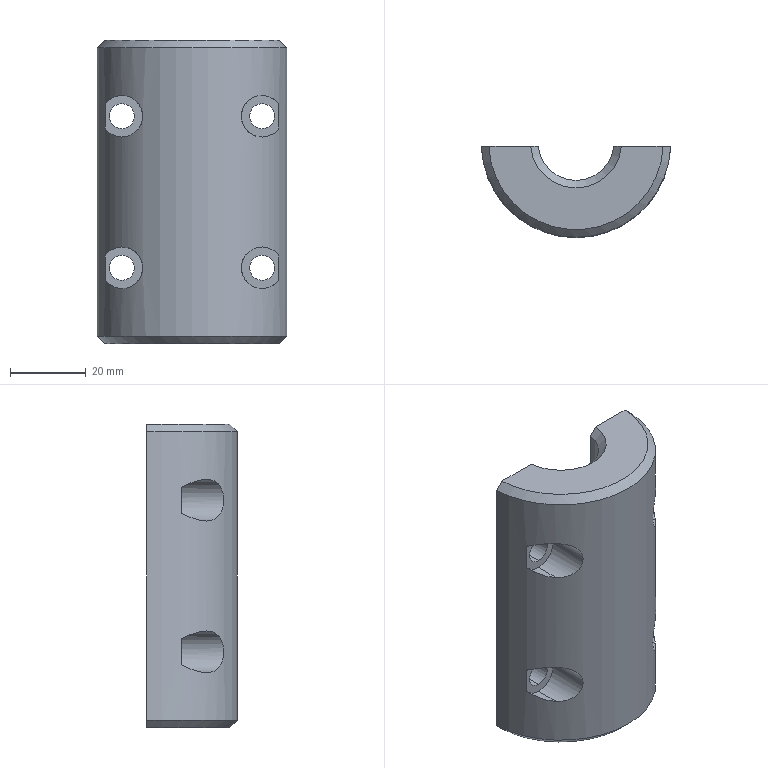Part | SolidWorks | features Chamfer 1, Extrusion 1, HoleWzd 1, ICE 1 | 1 solid | 34 faces | box 49.96 x 24 x 80 mm | volume 59562 mm3 | cylinder 22 | plane 8 | cone 4 | commonest cylinder face diameters 11 x12 6.6 x8 20 x1 50 x1
STEP:
#1=CARTESIAN_POINT('',(18.5,-1.,23.3));
#2=VERTEX_POINT('',#1);
#3=CARTESIAN_POINT('',(18.5,-1.,16.7));
#4=VERTEX_POINT('',#3);
#5=CARTESIAN_POINT('',(18.5,-1.,20.));
#6=DIRECTION('',(0.,-1.,0.));
#7=DIRECTION('',(0.,0.,-1.));
#8=AXIS2_PLACEMENT_3D('',#5,#6,#7);
#9=CIRCLE('',#8,3.3);
#10=EDGE_CURVE('',#2,#4,#9,.T.);
#11=ORIENTED_EDGE('',*,*,#10,.F.);
#12=CARTESIAN_POINT('',(18.5,-10.2,23.3));
#13=VERTEX_POINT('',#12);
#14=CARTESIAN_POINT('',(18.5,-17.,23.3));
#15=DIRECTION('',(0.,-1.,0.));
#16=VECTOR('',#15,1000.);
#17=LINE('',#14,#16);
#18=EDGE_CURVE('',#2,#13,#17,.T.);
#19=ORIENTED_EDGE('',*,*,#18,.T.);
#20=CARTESIAN_POINT('',(18.5,-10.2,16.7));
#21=VERTEX_POINT('',#20);
#22=CARTESIAN_POINT('',(18.5,-10.2,20.));
#23=DIRECTION('',(0.,-1.,0.));
#24=DIRECTION('',(0.,0.,-1.));
#25=AXIS2_PLACEMENT_3D('',#22,#23,#24);
#26=CIRCLE('',#25,3.3);
#27=EDGE_CURVE('',#13,#21,#26,.T.);
#28=ORIENTED_EDGE('',*,*,#27,.T.);
#29=CARTESIAN_POINT('',(18.5,-17.,16.7));
#30=DIRECTION('',(0.,-1.,0.));
#31=VECTOR('',#30,1000.);
#32=LINE('',#29,#31);
#33=EDGE_CURVE('',#4,#21,#32,.T.);
#34=ORIENTED_EDGE('',*,*,#33,.F.);
#35=EDGE_LOOP('',(#11,#19,#28,#34));
#36=FACE_OUTER_BOUND('',#35,.T.);
#37=CARTESIAN_POINT('',(18.5,-17.,20.));
#38=DIRECTION('',(0.,-1.,0.));
#39=DIRECTION('',(0.,0.,-1.));
#40=AXIS2_PLACEMENT_3D('',#37,#38,#39);
#41=CYLINDRICAL_SURFACE('',#40,3.3);
#42=ADVANCED_FACE('',(#36),#41,.F.);
#43=CARTESIAN_POINT('',(-18.5,-1.,23.3));
#44=VERTEX_POINT('',#43);
#45=CARTESIAN_POINT('',(-18.5,-1.,16.7));
#46=VERTEX_POINT('',#45);
#47=CARTESIAN_POINT('',(-18.5,-1.,20.));
#48=DIRECTION('',(0.,-1.,0.));
#49=DIRECTION('',(0.,0.,-1.));
#50=AXIS2_PLACEMENT_3D('',#47,#48,#49);
#51=CIRCLE('',#50,3.3);
#52=EDGE_CURVE('',#44,#46,#51,.T.);
#53=ORIENTED_EDGE('',*,*,#52,.F.);
#54=CARTESIAN_POINT('',(-18.5,-10.2,23.3));
#55=VERTEX_POINT('',#54);
#56=CARTESIAN_POINT('',(-18.5,-17.,23.3));
#57=DIRECTION('',(0.,-1.,0.));
#58=VECTOR('',#57,1000.);
#59=LINE('',#56,#58);
#60=EDGE_CURVE('',#44,#55,#59,.T.);
#61=ORIENTED_EDGE('',*,*,#60,.T.);
#62=CARTESIAN_POINT('',(-18.5,-10.2,16.7));
#63=VERTEX_POINT('',#62);
#64=CARTESIAN_POINT('',(-18.5,-10.2,20.));
#65=DIRECTION('',(0.,-1.,0.));
#66=DIRECTION('',(0.,0.,-1.));
#67=AXIS2_PLACEMENT_3D('',#64,#65,#66);
#68=CIRCLE('',#67,3.3);
#69=EDGE_CURVE('',#55,#63,#68,.T.);
#70=ORIENTED_EDGE('',*,*,#69,.T.);
#71=CARTESIAN_POINT('',(-18.5,-17.,16.7));
#72=DIRECTION('',(0.,-1.,0.));
#73=VECTOR('',#72,1000.);
#74=LINE('',#71,#73);
#75=EDGE_CURVE('',#46,#63,#74,.T.);
#76=ORIENTED_EDGE('',*,*,#75,.F.);
#77=EDGE_LOOP('',(#53,#61,#70,#76));
#78=FACE_OUTER_BOUND('',#77,.T.);
#79=CARTESIAN_POINT('',(-18.5,-17.,20.));
#80=DIRECTION('',(0.,-1.,0.));
#81=DIRECTION('',(0.,0.,-1.));
#82=AXIS2_PLACEMENT_3D('',#79,#80,#81);
#83=CYLINDRICAL_SURFACE('',#82,3.3);
#84=ADVANCED_FACE('',(#78),#83,.F.);
#85=CARTESIAN_POINT('',(-18.5,-1.,63.3));
#86=VERTEX_POINT('',#85);
#87=CARTESIAN_POINT('',(-18.5,-1.,56.7));
#88=VERTEX_POINT('',#87);
#89=CARTESIAN_POINT('',(-18.5,-1.,60.));
#90=DIRECTION('',(0.,-1.,0.));
#91=DIRECTION('',(0.,0.,-1.));
#92=AXIS2_PLACEMENT_3D('',#89,#90,#91);
#93=CIRCLE('',#92,3.3);
#94=EDGE_CURVE('',#86,#88,#93,.T.);
#95=ORIENTED_EDGE('',*,*,#94,.F.);
#96=CARTESIAN_POINT('',(-18.5,-10.2,63.3));
#97=VERTEX_POINT('',#96);
#98=CARTESIAN_POINT('',(-18.5,-17.,63.3));
#99=DIRECTION('',(0.,-1.,0.));
#100=VECTOR('',#99,1000.);
#101=LINE('',#98,#100);
#102=EDGE_CURVE('',#86,#97,#101,.T.);
#103=ORIENTED_EDGE('',*,*,#102,.T.);
#104=CARTESIAN_POINT('',(-18.5,-10.2,56.7));
#105=VERTEX_POINT('',#104);
#106=CARTESIAN_POINT('',(-18.5,-10.2,60.));
#107=DIRECTION('',(0.,-1.,0.));
#108=DIRECTION('',(0.,0.,-1.));
#109=AXIS2_PLACEMENT_3D('',#106,#107,#108);
#110=CIRCLE('',#109,3.3);
#111=EDGE_CURVE('',#97,#105,#110,.T.);
#112=ORIENTED_EDGE('',*,*,#111,.T.);
#113=CARTESIAN_POINT('',(-18.5,-17.,56.7));
#114=DIRECTION('',(0.,-1.,0.));
#115=VECTOR('',#114,1000.);
#116=LINE('',#113,#115);
#117=EDGE_CURVE('',#88,#105,#116,.T.);
#118=ORIENTED_EDGE('',*,*,#117,.F.);
#119=EDGE_LOOP('',(#95,#103,#112,#118));
#120=FACE_OUTER_BOUND('',#119,.T.);
#121=CARTESIAN_POINT('',(-18.5,-17.,60.));
#122=DIRECTION('',(0.,-1.,0.));
#123=DIRECTION('',(0.,0.,-1.));
#124=AXIS2_PLACEMENT_3D('',#121,#122,#123);
#125=CYLINDRICAL_SURFACE('',#124,3.3);
#126=ADVANCED_FACE('',(#120),#125,.F.);
#127=CARTESIAN_POINT('',(18.5,-1.,63.3));
#128=VERTEX_POINT('',#127);
#129=CARTESIAN_POINT('',(18.5,-1.,56.7));
#130=VERTEX_POINT('',#129);
#131=CARTESIAN_POINT('',(18.5,-1.,60.));
#132=DIRECTION('',(0.,-1.,0.));
#133=DIRECTION('',(0.,0.,-1.));
#134=AXIS2_PLACEMENT_3D('',#131,#132,#133);
#135=CIRCLE('',#134,3.3);
#136=EDGE_CURVE('',#128,#130,#135,.T.);
#137=ORIENTED_EDGE('',*,*,#136,.F.);
#138=CARTESIAN_POINT('',(18.5,-10.2,63.3));
#139=VERTEX_POINT('',#138);
#140=CARTESIAN_POINT('',(18.5,-17.,63.3));
#141=DIRECTION('',(0.,-1.,0.));
#142=VECTOR('',#141,1000.);
#143=LINE('',#140,#142);
#144=EDGE_CURVE('',#128,#139,#143,.T.);
#145=ORIENTED_EDGE('',*,*,#144,.T.);
#146=CARTESIAN_POINT('',(18.5,-10.2,56.7));
#147=VERTEX_POINT('',#146);
#148=CARTESIAN_POINT('',(18.5,-10.2,60.));
#149=DIRECTION('',(0.,-1.,0.));
#150=DIRECTION('',(0.,0.,-1.));
#151=AXIS2_PLACEMENT_3D('',#148,#149,#150);
#152=CIRCLE('',#151,3.3);
#153=EDGE_CURVE('',#139,#147,#152,.T.);
#154=ORIENTED_EDGE('',*,*,#153,.T.);
#155=CARTESIAN_POINT('',(18.5,-17.,56.7));
#156=DIRECTION('',(0.,-1.,0.));
#157=VECTOR('',#156,1000.);
#158=LINE('',#155,#157);
#159=EDGE_CURVE('',#130,#147,#158,.T.);
#160=ORIENTED_EDGE('',*,*,#159,.F.);
#161=EDGE_LOOP('',(#137,#145,#154,#160));
#162=FACE_OUTER_BOUND('',#161,.T.);
#163=CARTESIAN_POINT('',(18.5,-17.,60.));
#164=DIRECTION('',(0.,-1.,0.));
#165=DIRECTION('',(0.,0.,-1.));
#166=AXIS2_PLACEMENT_3D('',#163,#164,#165);
#167=CYLINDRICAL_SURFACE('',#166,3.3);
#168=ADVANCED_FACE('',(#162),#167,.F.);
#169=CARTESIAN_POINT('',(-18.5,-16.815,54.5));
#170=VERTEX_POINT('',#169);
#171=CARTESIAN_POINT('',(-22.825,-10.2,56.602));
#172=VERTEX_POINT('',#171);
#173=CARTESIAN_POINT('',(-18.5,-16.815,54.5));
#174=CARTESIAN_POINT('',(-18.967,-16.301,54.5));
#175=CARTESIAN_POINT('',(-19.407,-15.775,54.558));
#176=CARTESIAN_POINT('',(-20.028,-14.966,54.712));
#177=CARTESIAN_POINT('',(-20.229,-14.694,54.775));
#178=CARTESIAN_POINT('',(-20.618,-14.142,54.92));
#179=CARTESIAN_POINT('',(-20.808,-13.862,55.003));
#180=CARTESIAN_POINT('',(-21.352,-13.02,55.28));
#181=CARTESIAN_POINT('',(-21.685,-12.457,55.499));
#182=CARTESIAN_POINT('',(-22.295,-11.329,56.));
#183=CARTESIAN_POINT('',(-22.573,-10.763,56.281));
#184=CARTESIAN_POINT('',(-22.825,-10.2,56.602));
#185=B_SPLINE_CURVE_WITH_KNOTS('',3,(#173,#174,#175,#176,#177,#178,#179,#180,#181,#182,#183,#184),.UNSPECIFIED.,.F.,.F.,(4,2,2,2,2,4),(0.01974,0.02181,0.02284,0.02388,0.02594,0.02801),.UNSPECIFIED.);
#186=EDGE_CURVE('',#170,#172,#185,.T.);
#187=ORIENTED_EDGE('',*,*,#186,.F.);
#188=CARTESIAN_POINT('',(-18.5,-10.2,54.5));
#189=VERTEX_POINT('',#188);
#190=CARTESIAN_POINT('',(-18.5,-117.,54.5));
#191=DIRECTION('',(0.,1.,0.));
#192=VECTOR('',#191,1000.);
#193=LINE('',#190,#192);
#194=EDGE_CURVE('',#170,#189,#193,.T.);
#195=ORIENTED_EDGE('',*,*,#194,.T.);
#196=CARTESIAN_POINT('',(-18.5,-10.2,60.));
#197=DIRECTION('',(0.,-1.,0.));
#198=DIRECTION('',(0.,0.,-1.));
#199=AXIS2_PLACEMENT_3D('',#196,#197,#198);
#200=CIRCLE('',#199,5.5);
#201=EDGE_CURVE('',#172,#189,#200,.T.);
#202=ORIENTED_EDGE('',*,*,#201,.F.);
#203=EDGE_LOOP('',(#187,#195,#202));
#204=FACE_OUTER_BOUND('',#203,.T.);
#205=CARTESIAN_POINT('',(-18.5,-117.,60.));
#206=DIRECTION('',(0.,1.,0.));
#207=DIRECTION('',(0.,0.,1.));
#208=AXIS2_PLACEMENT_3D('',#205,#206,#207);
#209=CYLINDRICAL_SURFACE('',#208,5.5);
#210=ADVANCED_FACE('',(#204),#209,.F.);
#211=ORIENTED_EDGE('',*,*,#194,.F.);
#212=CARTESIAN_POINT('',(-18.5,-16.815,65.5));
#213=VERTEX_POINT('',#212);
#214=CARTESIAN_POINT('',(-18.5,-16.815,65.5));
#215=CARTESIAN_POINT('',(-18.218,-17.126,65.5));
#216=CARTESIAN_POINT('',(-17.927,-17.43,65.478));
#217=CARTESIAN_POINT('',(-17.34,-18.014,65.384));
#218=CARTESIAN_POINT('',(-17.042,-18.296,65.313));
#219=CARTESIAN_POINT('',(-16.439,-18.84,65.109));
#220=CARTESIAN_POINT('',(-16.133,-19.102,64.976));
#221=CARTESIAN_POINT('',(-15.538,-19.588,64.647));
#222=CARTESIAN_POINT('',(-15.248,-19.815,64.451));
#223=CARTESIAN_POINT('',(-14.828,-20.128,64.099));
#224=CARTESIAN_POINT('',(-14.691,-20.229,63.972));
#225=CARTESIAN_POINT('',(-14.429,-20.416,63.703));
#226=CARTESIAN_POINT('',(-14.304,-20.504,63.561));
#227=CARTESIAN_POINT('',(-14.066,-20.668,63.26));
#228=CARTESIAN_POINT('',(-13.953,-20.744,63.101));
#229=CARTESIAN_POINT('',(-13.741,-20.885,62.765));
#230=CARTESIAN_POINT('',(-13.643,-20.949,62.589));
#231=CARTESIAN_POINT('',(-13.379,-21.12,62.046));
#232=CARTESIAN_POINT('',(-13.241,-21.206,61.663));
#233=CARTESIAN_POINT('',(-13.098,-21.294,61.053));
#234=CARTESIAN_POINT('',(-13.061,-21.317,60.845));
#235=CARTESIAN_POINT('',(-13.013,-21.346,60.43));
#236=CARTESIAN_POINT('',(-13.001,-21.354,60.222));
#237=CARTESIAN_POINT('',(-12.999,-21.355,59.595));
#238=CARTESIAN_POINT('',(-13.047,-21.326,59.17));
#239=CARTESIAN_POINT('',(-13.187,-21.239,58.564));
#240=CARTESIAN_POINT('',(-13.244,-21.204,58.366));
#241=CARTESIAN_POINT('',(-13.381,-21.118,57.978));
#242=CARTESIAN_POINT('',(-13.461,-21.067,57.787));
#243=CARTESIAN_POINT('',(-13.725,-20.897,57.241));
#244=CARTESIAN_POINT('',(-13.936,-20.758,56.906));
#245=CARTESIAN_POINT('',(-14.417,-20.426,56.294));
#246=CARTESIAN_POINT('',(-14.68,-20.239,56.026));
#247=CARTESIAN_POINT('',(-15.098,-19.927,55.674));
#248=CARTESIAN_POINT('',(-15.242,-19.817,55.565));
#249=CARTESIAN_POINT('',(-15.534,-19.589,55.365));
#250=CARTESIAN_POINT('',(-15.682,-19.471,55.274));
#251=CARTESIAN_POINT('',(-16.127,-19.107,55.027));
#252=CARTESIAN_POINT('',(-16.427,-18.85,54.895));
#253=CARTESIAN_POINT('',(-17.032,-18.305,54.69));
#254=CARTESIAN_POINT('',(-17.335,-18.019,54.617));
#255=CARTESIAN_POINT('',(-17.926,-17.431,54.522));
#256=CARTESIAN_POINT('',(-18.217,-17.126,54.5));
#257=CARTESIAN_POINT('',(-18.5,-16.815,54.5));
#258=B_SPLINE_CURVE_WITH_KNOTS('',3,(#214,#215,#216,#217,#218,#219,#220,#221,#222,#223,#224,#225,#226,#227,#228,#229,#230,#231,#232,#233,#234,#235,#236,#237,#238,#239,#240,#241,#242,#243,#244,#245,#246,#247,#248,#249,#250,#251,#252,#253,#254,#255,#256,#257),.UNSPECIFIED.,.F.,.F.,(4,2,2,2,2,2,2,2,2,2,2,2,2,2,2,2,2,2,2,2,2,4),(-0.0002486,0.001001,0.00225,0.0035,0.004749,0.005374,0.005999,0.006623,0.007248,0.008497,0.009122,0.009747,0.011,0.01162,0.01225,0.0135,0.01474,0.01537,0.01599,0.01724,0.01849,0.01974),.UNSPECIFIED.);
#259=EDGE_CURVE('',#213,#170,#258,.T.);
#260=ORIENTED_EDGE('',*,*,#259,.F.);
#261=CARTESIAN_POINT('',(-18.5,-10.2,65.5));
#262=VERTEX_POINT('',#261);
#263=CARTESIAN_POINT('',(-18.5,-117.,65.5));
#264=DIRECTION('',(0.,1.,0.));
#265=VECTOR('',#264,1000.);
#266=LINE('',#263,#265);
#267=EDGE_CURVE('',#213,#262,#266,.T.);
#268=ORIENTED_EDGE('',*,*,#267,.T.);
#269=CARTESIAN_POINT('',(-18.5,-10.2,60.));
#270=DIRECTION('',(0.,-1.,0.));
#271=DIRECTION('',(0.,0.,-1.));
#272=AXIS2_PLACEMENT_3D('',#269,#270,#271);
#273=CIRCLE('',#272,5.5);
#274=EDGE_CURVE('',#189,#262,#273,.T.);
#275=ORIENTED_EDGE('',*,*,#274,.F.);
#276=EDGE_LOOP('',(#211,#260,#268,#275));
#277=FACE_OUTER_BOUND('',#276,.T.);
#278=CARTESIAN_POINT('',(-18.5,-117.,60.));
#279=DIRECTION('',(0.,1.,0.));
#280=DIRECTION('',(0.,0.,1.));
#281=AXIS2_PLACEMENT_3D('',#278,#279,#280);
#282=CYLINDRICAL_SURFACE('',#281,5.5);
#283=ADVANCED_FACE('',(#277),#282,.F.);
#284=CARTESIAN_POINT('',(18.5,-16.815,54.5));
#285=VERTEX_POINT('',#284);
#286=CARTESIAN_POINT('',(18.5,-16.815,65.5));
#287=VERTEX_POINT('',#286);
#288=CARTESIAN_POINT('',(18.5,-16.815,54.5));
#289=CARTESIAN_POINT('',(18.218,-17.126,54.5));
#290=CARTESIAN_POINT('',(17.927,-17.43,54.522));
#291=CARTESIAN_POINT('',(17.34,-18.014,54.616));
#292=CARTESIAN_POINT('',(17.042,-18.296,54.687));
#293=CARTESIAN_POINT('',(16.439,-18.84,54.891));
#294=CARTESIAN_POINT('',(16.133,-19.102,55.024));
#295=CARTESIAN_POINT('',(15.538,-19.588,55.353));
#296=CARTESIAN_POINT('',(15.248,-19.815,55.549));
#297=CARTESIAN_POINT('',(14.828,-20.128,55.901));
#298=CARTESIAN_POINT('',(14.691,-20.229,56.028));
#299=CARTESIAN_POINT('',(14.429,-20.416,56.297));
#300=CARTESIAN_POINT('',(14.304,-20.504,56.439));
#301=CARTESIAN_POINT('',(14.066,-20.668,56.74));
#302=CARTESIAN_POINT('',(13.953,-20.744,56.899));
#303=CARTESIAN_POINT('',(13.741,-20.885,57.235));
#304=CARTESIAN_POINT('',(13.643,-20.949,57.411));
#305=CARTESIAN_POINT('',(13.379,-21.12,57.954));
#306=CARTESIAN_POINT('',(13.241,-21.206,58.337));
#307=CARTESIAN_POINT('',(13.098,-21.294,58.947));
#308=CARTESIAN_POINT('',(13.061,-21.317,59.155));
#309=CARTESIAN_POINT('',(13.013,-21.346,59.57));
#310=CARTESIAN_POINT('',(13.001,-21.354,59.778));
#311=CARTESIAN_POINT('',(12.999,-21.355,60.405));
#312=CARTESIAN_POINT('',(13.047,-21.326,60.83));
#313=CARTESIAN_POINT('',(13.187,-21.239,61.436));
#314=CARTESIAN_POINT('',(13.244,-21.204,61.634));
#315=CARTESIAN_POINT('',(13.381,-21.118,62.022));
#316=CARTESIAN_POINT('',(13.461,-21.067,62.213));
#317=CARTESIAN_POINT('',(13.725,-20.897,62.759));
#318=CARTESIAN_POINT('',(13.936,-20.758,63.094));
#319=CARTESIAN_POINT('',(14.417,-20.426,63.706));
#320=CARTESIAN_POINT('',(14.68,-20.239,63.974));
#321=CARTESIAN_POINT('',(15.098,-19.927,64.326));
#322=CARTESIAN_POINT('',(15.242,-19.817,64.435));
#323=CARTESIAN_POINT('',(15.534,-19.589,64.635));
#324=CARTESIAN_POINT('',(15.682,-19.471,64.726));
#325=CARTESIAN_POINT('',(16.127,-19.107,64.973));
#326=CARTESIAN_POINT('',(16.427,-18.85,65.105));
#327=CARTESIAN_POINT('',(17.032,-18.305,65.31));
#328=CARTESIAN_POINT('',(17.335,-18.019,65.383));
#329=CARTESIAN_POINT('',(17.926,-17.431,65.478));
#330=CARTESIAN_POINT('',(18.217,-17.126,65.5));
#331=CARTESIAN_POINT('',(18.5,-16.815,65.5));
#332=B_SPLINE_CURVE_WITH_KNOTS('',3,(#288,#289,#290,#291,#292,#293,#294,#295,#296,#297,#298,#299,#300,#301,#302,#303,#304,#305,#306,#307,#308,#309,#310,#311,#312,#313,#314,#315,#316,#317,#318,#319,#320,#321,#322,#323,#324,#325,#326,#327,#328,#329,#330,#331),.UNSPECIFIED.,.F.,.F.,(4,2,2,2,2,2,2,2,2,2,2,2,2,2,2,2,2,2,2,2,2,4),(-0.0002486,0.001001,0.00225,0.0035,0.004749,0.005374,0.005999,0.006623,0.007248,0.008497,0.009122,0.009747,0.011,0.01162,0.01225,0.0135,0.01474,0.01537,0.01599,0.01724,0.01849,0.01974),.UNSPECIFIED.);
#333=EDGE_CURVE('',#285,#287,#332,.T.);
#334=ORIENTED_EDGE('',*,*,#333,.F.);
#335=CARTESIAN_POINT('',(18.5,-10.2,54.5));
#336=VERTEX_POINT('',#335);
#337=CARTESIAN_POINT('',(18.5,-117.,54.5));
#338=DIRECTION('',(0.,1.,0.));
#339=VECTOR('',#338,1000.);
#340=LINE('',#337,#339);
#341=EDGE_CURVE('',#285,#336,#340,.T.);
#342=ORIENTED_EDGE('',*,*,#341,.T.);
#343=CARTESIAN_POINT('',(18.5,-10.2,65.5));
#344=VERTEX_POINT('',#343);
#345=CARTESIAN_POINT('',(18.5,-10.2,60.));
#346=DIRECTION('',(0.,-1.,0.));
#347=DIRECTION('',(0.,0.,-1.));
#348=AXIS2_PLACEMENT_3D('',#345,#346,#347);
#349=CIRCLE('',#348,5.5);
#350=EDGE_CURVE('',#344,#336,#349,.T.);
#351=ORIENTED_EDGE('',*,*,#350,.F.);
#352=CARTESIAN_POINT('',(18.5,-117.,65.5));
#353=DIRECTION('',(0.,1.,0.));
#354=VECTOR('',#353,1000.);
#355=LINE('',#352,#354);
#356=EDGE_CURVE('',#287,#344,#355,.T.);
#357=ORIENTED_EDGE('',*,*,#356,.F.);
#358=EDGE_LOOP('',(#334,#342,#351,#357));
#359=FACE_OUTER_BOUND('',#358,.T.);
#360=CARTESIAN_POINT('',(18.5,-117.,60.));
#361=DIRECTION('',(0.,1.,0.));
#362=DIRECTION('',(0.,0.,1.));
#363=AXIS2_PLACEMENT_3D('',#360,#361,#362);
#364=CYLINDRICAL_SURFACE('',#363,5.5);
#365=ADVANCED_FACE('',(#359),#364,.F.);
#366=CARTESIAN_POINT('',(22.825,-10.2,63.398));
#367=VERTEX_POINT('',#366);
#368=CARTESIAN_POINT('',(18.5,-16.815,65.5));
#369=CARTESIAN_POINT('',(18.967,-16.301,65.5));
#370=CARTESIAN_POINT('',(19.407,-15.775,65.442));
#371=CARTESIAN_POINT('',(20.028,-14.966,65.288));
#372=CARTESIAN_POINT('',(20.229,-14.694,65.225));
#373=CARTESIAN_POINT('',(20.618,-14.142,65.08));
#374=CARTESIAN_POINT('',(20.808,-13.862,64.997));
#375=CARTESIAN_POINT('',(21.352,-13.02,64.72));
#376=CARTESIAN_POINT('',(21.685,-12.457,64.501));
#377=CARTESIAN_POINT('',(22.295,-11.329,64.));
#378=CARTESIAN_POINT('',(22.573,-10.763,63.719));
#379=CARTESIAN_POINT('',(22.825,-10.2,63.398));
#380=B_SPLINE_CURVE_WITH_KNOTS('',3,(#368,#369,#370,#371,#372,#373,#374,#375,#376,#377,#378,#379),.UNSPECIFIED.,.F.,.F.,(4,2,2,2,2,4),(0.01974,0.02181,0.02284,0.02388,0.02594,0.02801),.UNSPECIFIED.);
#381=EDGE_CURVE('',#287,#367,#380,.T.);
#382=ORIENTED_EDGE('',*,*,#381,.F.);
#383=ORIENTED_EDGE('',*,*,#356,.T.);
#384=CARTESIAN_POINT('',(18.5,-10.2,60.));
#385=DIRECTION('',(0.,-1.,0.));
#386=DIRECTION('',(0.,0.,-1.));
#387=AXIS2_PLACEMENT_3D('',#384,#385,#386);
#388=CIRCLE('',#387,5.5);
#389=EDGE_CURVE('',#367,#344,#388,.T.);
#390=ORIENTED_EDGE('',*,*,#389,.F.);
#391=EDGE_LOOP('',(#382,#383,#390));
#392=FACE_OUTER_BOUND('',#391,.T.);
#393=CARTESIAN_POINT('',(18.5,-117.,60.));
#394=DIRECTION('',(0.,1.,0.));
#395=DIRECTION('',(0.,0.,1.));
#396=AXIS2_PLACEMENT_3D('',#393,#394,#395);
#397=CYLINDRICAL_SURFACE('',#396,5.5);
#398=ADVANCED_FACE('',(#392),#397,.F.);
#399=CARTESIAN_POINT('',(18.5,-16.815,14.5));
#400=VERTEX_POINT('',#399);
#401=CARTESIAN_POINT('',(18.5,-16.815,25.5));
#402=VERTEX_POINT('',#401);
#403=CARTESIAN_POINT('',(18.5,-16.815,14.5));
#404=CARTESIAN_POINT('',(18.218,-17.126,14.5));
#405=CARTESIAN_POINT('',(17.927,-17.43,14.522));
#406=CARTESIAN_POINT('',(17.34,-18.014,14.616));
#407=CARTESIAN_POINT('',(17.042,-18.296,14.687));
#408=CARTESIAN_POINT('',(16.439,-18.84,14.891));
#409=CARTESIAN_POINT('',(16.133,-19.102,15.024));
#410=CARTESIAN_POINT('',(15.538,-19.588,15.353));
#411=CARTESIAN_POINT('',(15.248,-19.815,15.549));
#412=CARTESIAN_POINT('',(14.828,-20.128,15.901));
#413=CARTESIAN_POINT('',(14.691,-20.229,16.028));
#414=CARTESIAN_POINT('',(14.429,-20.416,16.297));
#415=CARTESIAN_POINT('',(14.304,-20.504,16.439));
#416=CARTESIAN_POINT('',(14.066,-20.668,16.74));
#417=CARTESIAN_POINT('',(13.953,-20.744,16.899));
#418=CARTESIAN_POINT('',(13.741,-20.885,17.235));
#419=CARTESIAN_POINT('',(13.643,-20.949,17.411));
#420=CARTESIAN_POINT('',(13.379,-21.12,17.954));
#421=CARTESIAN_POINT('',(13.241,-21.206,18.337));
#422=CARTESIAN_POINT('',(13.098,-21.294,18.947));
#423=CARTESIAN_POINT('',(13.061,-21.317,19.155));
#424=CARTESIAN_POINT('',(13.013,-21.346,19.57));
#425=CARTESIAN_POINT('',(13.001,-21.354,19.778));
#426=CARTESIAN_POINT('',(12.999,-21.355,20.405));
#427=CARTESIAN_POINT('',(13.047,-21.326,20.83));
#428=CARTESIAN_POINT('',(13.187,-21.239,21.436));
#429=CARTESIAN_POINT('',(13.244,-21.204,21.634));
#430=CARTESIAN_POINT('',(13.381,-21.118,22.022));
#431=CARTESIAN_POINT('',(13.461,-21.067,22.213));
#432=CARTESIAN_POINT('',(13.725,-20.897,22.759));
#433=CARTESIAN_POINT('',(13.936,-20.758,23.094));
#434=CARTESIAN_POINT('',(14.417,-20.426,23.706));
#435=CARTESIAN_POINT('',(14.68,-20.239,23.974));
#436=CARTESIAN_POINT('',(15.098,-19.927,24.326));
#437=CARTESIAN_POINT('',(15.242,-19.817,24.435));
#438=CARTESIAN_POINT('',(15.534,-19.589,24.635));
#439=CARTESIAN_POINT('',(15.682,-19.471,24.726));
#440=CARTESIAN_POINT('',(16.127,-19.107,24.973));
#441=CARTESIAN_POINT('',(16.427,-18.85,25.105));
#442=CARTESIAN_POINT('',(17.032,-18.305,25.31));
#443=CARTESIAN_POINT('',(17.335,-18.019,25.383));
#444=CARTESIAN_POINT('',(17.926,-17.431,25.478));
#445=CARTESIAN_POINT('',(18.217,-17.126,25.5));
#446=CARTESIAN_POINT('',(18.5,-16.815,25.5));
#447=B_SPLINE_CURVE_WITH_KNOTS('',3,(#403,#404,#405,#406,#407,#408,#409,#410,#411,#412,#413,#414,#415,#416,#417,#418,#419,#420,#421,#422,#423,#424,#425,#426,#427,#428,#429,#430,#431,#432,#433,#434,#435,#436,#437,#438,#439,#440,#441,#442,#443,#444,#445,#446),.UNSPECIFIED.,.F.,.F.,(4,2,2,2,2,2,2,2,2,2,2,2,2,2,2,2,2,2,2,2,2,4),(-0.0002486,0.001001,0.00225,0.0035,0.004749,0.005374,0.005999,0.006623,0.007248,0.008497,0.009122,0.009747,0.011,0.01162,0.01225,0.0135,0.01474,0.01537,0.01599,0.01724,0.01849,0.01974),.UNSPECIFIED.);
#448=EDGE_CURVE('',#400,#402,#447,.T.);
#449=ORIENTED_EDGE('',*,*,#448,.F.);
#450=CARTESIAN_POINT('',(18.5,-10.2,14.5));
#451=VERTEX_POINT('',#450);
#452=CARTESIAN_POINT('',(18.5,-117.,14.5));
#453=DIRECTION('',(0.,1.,0.));
#454=VECTOR('',#453,1000.);
#455=LINE('',#452,#454);
#456=EDGE_CURVE('',#400,#451,#455,.T.);
#457=ORIENTED_EDGE('',*,*,#456,.T.);
#458=CARTESIAN_POINT('',(18.5,-10.2,25.5));
#459=VERTEX_POINT('',#458);
#460=CARTESIAN_POINT('',(18.5,-10.2,20.));
#461=DIRECTION('',(0.,-1.,0.));
#462=DIRECTION('',(0.,0.,-1.));
#463=AXIS2_PLACEMENT_3D('',#460,#461,#462);
#464=CIRCLE('',#463,5.5);
#465=EDGE_CURVE('',#459,#451,#464,.T.);
#466=ORIENTED_EDGE('',*,*,#465,.F.);
#467=CARTESIAN_POINT('',(18.5,-117.,25.5));
#468=DIRECTION('',(0.,1.,0.));
#469=VECTOR('',#468,1000.);
#470=LINE('',#467,#469);
#471=EDGE_CURVE('',#402,#459,#470,.T.);
#472=ORIENTED_EDGE('',*,*,#471,.F.);
#473=EDGE_LOOP('',(#449,#457,#466,#472));
#474=FACE_OUTER_BOUND('',#473,.T.);
#475=CARTESIAN_POINT('',(18.5,-117.,20.));
#476=DIRECTION('',(0.,1.,0.));
#477=DIRECTION('',(0.,0.,1.));
#478=AXIS2_PLACEMENT_3D('',#475,#476,#477);
#479=CYLINDRICAL_SURFACE('',#478,5.5);
#480=ADVANCED_FACE('',(#474),#479,.F.);
#481=CARTESIAN_POINT('',(22.825,-10.2,23.398));
#482=VERTEX_POINT('',#481);
#483=CARTESIAN_POINT('',(18.5,-16.815,25.5));
#484=CARTESIAN_POINT('',(18.967,-16.301,25.5));
#485=CARTESIAN_POINT('',(19.407,-15.775,25.442));
#486=CARTESIAN_POINT('',(20.028,-14.966,25.288));
#487=CARTESIAN_POINT('',(20.229,-14.694,25.225));
#488=CARTESIAN_POINT('',(20.618,-14.142,25.08));
#489=CARTESIAN_POINT('',(20.808,-13.862,24.997));
#490=CARTESIAN_POINT('',(21.352,-13.02,24.72));
#491=CARTESIAN_POINT('',(21.685,-12.457,24.501));
#492=CARTESIAN_POINT('',(22.295,-11.329,24.));
#493=CARTESIAN_POINT('',(22.573,-10.763,23.719));
#494=CARTESIAN_POINT('',(22.825,-10.2,23.398));
#495=B_SPLINE_CURVE_WITH_KNOTS('',3,(#483,#484,#485,#486,#487,#488,#489,#490,#491,#492,#493,#494),.UNSPECIFIED.,.F.,.F.,(4,2,2,2,2,4),(0.01974,0.02181,0.02284,0.02388,0.02594,0.02801),.UNSPECIFIED.);
#496=EDGE_CURVE('',#402,#482,#495,.T.);
#497=ORIENTED_EDGE('',*,*,#496,.F.);
#498=ORIENTED_EDGE('',*,*,#471,.T.);
#499=CARTESIAN_POINT('',(18.5,-10.2,20.));
#500=DIRECTION('',(0.,-1.,0.));
#501=DIRECTION('',(0.,0.,-1.));
#502=AXIS2_PLACEMENT_3D('',#499,#500,#501);
#503=CIRCLE('',#502,5.5);
#504=EDGE_CURVE('',#482,#459,#503,.T.);
#505=ORIENTED_EDGE('',*,*,#504,.F.);
#506=EDGE_LOOP('',(#497,#498,#505));
#507=FACE_OUTER_BOUND('',#506,.T.);
#508=CARTESIAN_POINT('',(18.5,-117.,20.));
#509=DIRECTION('',(0.,1.,0.));
#510=DIRECTION('',(0.,0.,1.));
#511=AXIS2_PLACEMENT_3D('',#508,#509,#510);
#512=CYLINDRICAL_SURFACE('',#511,5.5);
#513=ADVANCED_FACE('',(#507),#512,.F.);
#514=CARTESIAN_POINT('',(-18.5,-16.815,14.5));
#515=VERTEX_POINT('',#514);
#516=CARTESIAN_POINT('',(-22.825,-10.2,16.602));
#517=VERTEX_POINT('',#516);
#518=CARTESIAN_POINT('',(-18.5,-16.815,14.5));
#519=CARTESIAN_POINT('',(-18.967,-16.301,14.5));
#520=CARTESIAN_POINT('',(-19.407,-15.775,14.558));
#521=CARTESIAN_POINT('',(-20.028,-14.966,14.712));
#522=CARTESIAN_POINT('',(-20.229,-14.694,14.775));
#523=CARTESIAN_POINT('',(-20.618,-14.142,14.92));
#524=CARTESIAN_POINT('',(-20.808,-13.862,15.003));
#525=CARTESIAN_POINT('',(-21.352,-13.02,15.28));
#526=CARTESIAN_POINT('',(-21.685,-12.457,15.499));
#527=CARTESIAN_POINT('',(-22.295,-11.329,16.));
#528=CARTESIAN_POINT('',(-22.573,-10.763,16.281));
#529=CARTESIAN_POINT('',(-22.825,-10.2,16.602));
#530=B_SPLINE_CURVE_WITH_KNOTS('',3,(#518,#519,#520,#521,#522,#523,#524,#525,#526,#527,#528,#529),.UNSPECIFIED.,.F.,.F.,(4,2,2,2,2,4),(0.01974,0.02181,0.02284,0.02388,0.02594,0.02801),.UNSPECIFIED.);
#531=EDGE_CURVE('',#515,#517,#530,.T.);
#532=ORIENTED_EDGE('',*,*,#531,.F.);
#533=CARTESIAN_POINT('',(-18.5,-10.2,14.5));
#534=VERTEX_POINT('',#533);
#535=CARTESIAN_POINT('',(-18.5,-117.,14.5));
#536=DIRECTION('',(0.,1.,0.));
#537=VECTOR('',#536,1000.);
#538=LINE('',#535,#537);
#539=EDGE_CURVE('',#515,#534,#538,.T.);
#540=ORIENTED_EDGE('',*,*,#539,.T.);
#541=CARTESIAN_POINT('',(-18.5,-10.2,20.));
#542=DIRECTION('',(0.,-1.,0.));
#543=DIRECTION('',(0.,0.,-1.));
#544=AXIS2_PLACEMENT_3D('',#541,#542,#543);
#545=CIRCLE('',#544,5.5);
#546=EDGE_CURVE('',#517,#534,#545,.T.);
#547=ORIENTED_EDGE('',*,*,#546,.F.);
#548=EDGE_LOOP('',(#532,#540,#547));
#549=FACE_OUTER_BOUND('',#548,.T.);
#550=CARTESIAN_POINT('',(-18.5,-117.,20.));
#551=DIRECTION('',(0.,1.,0.));
#552=DIRECTION('',(0.,0.,1.));
#553=AXIS2_PLACEMENT_3D('',#550,#551,#552);
#554=CYLINDRICAL_SURFACE('',#553,5.5);
#555=ADVANCED_FACE('',(#549),#554,.F.);
#556=ORIENTED_EDGE('',*,*,#539,.F.);
#557=CARTESIAN_POINT('',(-18.5,-16.815,25.5));
#558=VERTEX_POINT('',#557);
#559=CARTESIAN_POINT('',(-18.5,-16.815,25.5));
#560=CARTESIAN_POINT('',(-18.218,-17.126,25.5));
#561=CARTESIAN_POINT('',(-17.927,-17.43,25.478));
#562=CARTESIAN_POINT('',(-17.34,-18.014,25.384));
#563=CARTESIAN_POINT('',(-17.042,-18.296,25.313));
#564=CARTESIAN_POINT('',(-16.439,-18.84,25.109));
#565=CARTESIAN_POINT('',(-16.133,-19.102,24.976));
#566=CARTESIAN_POINT('',(-15.538,-19.588,24.647));
#567=CARTESIAN_POINT('',(-15.248,-19.815,24.451));
#568=CARTESIAN_POINT('',(-14.828,-20.128,24.099));
#569=CARTESIAN_POINT('',(-14.691,-20.229,23.972));
#570=CARTESIAN_POINT('',(-14.429,-20.416,23.703));
#571=CARTESIAN_POINT('',(-14.304,-20.504,23.561));
#572=CARTESIAN_POINT('',(-14.066,-20.668,23.26));
#573=CARTESIAN_POINT('',(-13.953,-20.744,23.101));
#574=CARTESIAN_POINT('',(-13.741,-20.885,22.765));
#575=CARTESIAN_POINT('',(-13.643,-20.949,22.589));
#576=CARTESIAN_POINT('',(-13.379,-21.12,22.046));
#577=CARTESIAN_POINT('',(-13.241,-21.206,21.663));
#578=CARTESIAN_POINT('',(-13.098,-21.294,21.053));
#579=CARTESIAN_POINT('',(-13.061,-21.317,20.845));
#580=CARTESIAN_POINT('',(-13.013,-21.346,20.43));
#581=CARTESIAN_POINT('',(-13.001,-21.354,20.222));
#582=CARTESIAN_POINT('',(-12.999,-21.355,19.595));
#583=CARTESIAN_POINT('',(-13.047,-21.326,19.17));
#584=CARTESIAN_POINT('',(-13.187,-21.239,18.564));
#585=CARTESIAN_POINT('',(-13.244,-21.204,18.366));
#586=CARTESIAN_POINT('',(-13.381,-21.118,17.978));
#587=CARTESIAN_POINT('',(-13.461,-21.067,17.787));
#588=CARTESIAN_POINT('',(-13.725,-20.897,17.241));
#589=CARTESIAN_POINT('',(-13.936,-20.758,16.906));
#590=CARTESIAN_POINT('',(-14.417,-20.426,16.294));
#591=CARTESIAN_POINT('',(-14.68,-20.239,16.026));
#592=CARTESIAN_POINT('',(-15.098,-19.927,15.674));
#593=CARTESIAN_POINT('',(-15.242,-19.817,15.565));
#594=CARTESIAN_POINT('',(-15.534,-19.589,15.365));
#595=CARTESIAN_POINT('',(-15.682,-19.471,15.274));
#596=CARTESIAN_POINT('',(-16.127,-19.107,15.027));
#597=CARTESIAN_POINT('',(-16.427,-18.85,14.895));
#598=CARTESIAN_POINT('',(-17.032,-18.305,14.69));
#599=CARTESIAN_POINT('',(-17.335,-18.019,14.617));
#600=CARTESIAN_POINT('',(-17.926,-17.431,14.522));
#601=CARTESIAN_POINT('',(-18.217,-17.126,14.5));
#602=CARTESIAN_POINT('',(-18.5,-16.815,14.5));
#603=B_SPLINE_CURVE_WITH_KNOTS('',3,(#559,#560,#561,#562,#563,#564,#565,#566,#567,#568,#569,#570,#571,#572,#573,#574,#575,#576,#577,#578,#579,#580,#581,#582,#583,#584,#585,#586,#587,#588,#589,#590,#591,#592,#593,#594,#595,#596,#597,#598,#599,#600,#601,#602),.UNSPECIFIED.,.F.,.F.,(4,2,2,2,2,2,2,2,2,2,2,2,2,2,2,2,2,2,2,2,2,4),(-0.0002486,0.001001,0.00225,0.0035,0.004749,0.005374,0.005999,0.006623,0.007248,0.008497,0.009122,0.009747,0.011,0.01162,0.01225,0.0135,0.01474,0.01537,0.01599,0.01724,0.01849,0.01974),.UNSPECIFIED.);
#604=EDGE_CURVE('',#558,#515,#603,.T.);
#605=ORIENTED_EDGE('',*,*,#604,.F.);
#606=CARTESIAN_POINT('',(-18.5,-10.2,25.5));
#607=VERTEX_POINT('',#606);
#608=CARTESIAN_POINT('',(-18.5,-117.,25.5));
#609=DIRECTION('',(0.,1.,0.));
#610=VECTOR('',#609,1000.);
#611=LINE('',#608,#610);
#612=EDGE_CURVE('',#558,#607,#611,.T.);
#613=ORIENTED_EDGE('',*,*,#612,.T.);
#614=CARTESIAN_POINT('',(-18.5,-10.2,20.));
#615=DIRECTION('',(0.,-1.,0.));
#616=DIRECTION('',(0.,0.,-1.));
#617=AXIS2_PLACEMENT_3D('',#614,#615,#616);
#618=CIRCLE('',#617,5.5);
#619=EDGE_CURVE('',#534,#607,#618,.T.);
#620=ORIENTED_EDGE('',*,*,#619,.F.);
#621=EDGE_LOOP('',(#556,#605,#613,#620));
#622=FACE_OUTER_BOUND('',#621,.T.);
#623=CARTESIAN_POINT('',(-18.5,-117.,20.));
#624=DIRECTION('',(0.,1.,0.));
#625=DIRECTION('',(0.,0.,1.));
#626=AXIS2_PLACEMENT_3D('',#623,#624,#625);
#627=CYLINDRICAL_SURFACE('',#626,5.5);
#628=ADVANCED_FACE('',(#622),#627,.F.);
#629=CARTESIAN_POINT('',(9.95,-1.,78.));
#630=VERTEX_POINT('',#629);
#631=CARTESIAN_POINT('',(9.95,-1.,2.));
#632=VERTEX_POINT('',#631);
#633=CARTESIAN_POINT('',(9.95,-1.,80.));
#634=DIRECTION('',(0.,0.,-1.));
#635=VECTOR('',#634,1000.);
#636=LINE('',#633,#635);
#637=EDGE_CURVE('',#630,#632,#636,.T.);
#638=ORIENTED_EDGE('',*,*,#637,.T.);
#639=CARTESIAN_POINT('',(-9.95,-1.,2.));
#640=VERTEX_POINT('',#639);
#641=CARTESIAN_POINT('',(0.,0.,2.));
#642=DIRECTION('',(0.,0.,-1.));
#643=DIRECTION('',(1.,0.,0.));
#644=AXIS2_PLACEMENT_3D('',#641,#642,#643);
#645=CIRCLE('',#644,10.);
#646=EDGE_CURVE('',#632,#640,#645,.T.);
#647=ORIENTED_EDGE('',*,*,#646,.T.);
#648=CARTESIAN_POINT('',(-9.95,-1.,78.));
#649=VERTEX_POINT('',#648);
#650=CARTESIAN_POINT('',(-9.95,-1.,80.));
#651=DIRECTION('',(0.,0.,-1.));
#652=VECTOR('',#651,1000.);
#653=LINE('',#650,#652);
#654=EDGE_CURVE('',#649,#640,#653,.T.);
#655=ORIENTED_EDGE('',*,*,#654,.F.);
#656=CARTESIAN_POINT('',(0.,0.,78.));
#657=DIRECTION('',(0.,0.,1.));
#658=DIRECTION('',(1.,0.,0.));
#659=AXIS2_PLACEMENT_3D('',#656,#657,#658);
#660=CIRCLE('',#659,10.);
#661=EDGE_CURVE('',#649,#630,#660,.T.);
#662=ORIENTED_EDGE('',*,*,#661,.T.);
#663=EDGE_LOOP('',(#638,#647,#655,#662));
#664=FACE_OUTER_BOUND('',#663,.T.);
#665=CARTESIAN_POINT('',(0.,0.,80.));
#666=DIRECTION('',(0.,0.,-1.));
#667=DIRECTION('',(-1.,0.,0.));
#668=AXIS2_PLACEMENT_3D('',#665,#666,#667);
#669=CYLINDRICAL_SURFACE('',#668,10.);
#670=ADVANCED_FACE('',(#664),#669,.F.);
#671=CARTESIAN_POINT('',(-18.5,-1.,20.));
#672=DIRECTION('',(0.,-1.,0.));
#673=DIRECTION('',(0.,0.,-1.));
#674=AXIS2_PLACEMENT_3D('',#671,#672,#673);
#675=CIRCLE('',#674,3.3);
#676=EDGE_CURVE('',#46,#44,#675,.T.);
#677=ORIENTED_EDGE('',*,*,#676,.T.);
#678=ORIENTED_EDGE('',*,*,#52,.T.);
#679=EDGE_LOOP('',(#677,#678));
#680=FACE_BOUND('',#679,.T.);
#681=CARTESIAN_POINT('',(-18.5,-1.,60.));
#682=DIRECTION('',(0.,-1.,0.));
#683=DIRECTION('',(0.,0.,-1.));
#684=AXIS2_PLACEMENT_3D('',#681,#682,#683);
#685=CIRCLE('',#684,3.3);
#686=EDGE_CURVE('',#88,#86,#685,.T.);
#687=ORIENTED_EDGE('',*,*,#686,.T.);
#688=ORIENTED_EDGE('',*,*,#94,.T.);
#689=EDGE_LOOP('',(#687,#688));
#690=FACE_BOUND('',#689,.T.);
#691=CARTESIAN_POINT('',(-11.958,-1.,0.));
#692=VERTEX_POINT('',#691);
#693=CARTESIAN_POINT('',(-22.978,-1.,0.));
#694=VERTEX_POINT('',#693);
#695=CARTESIAN_POINT('',(-24.98,-1.,0.));
#696=DIRECTION('',(-1.,0.,0.));
#697=VECTOR('',#696,1000.);
#698=LINE('',#695,#697);
#699=EDGE_CURVE('',#692,#694,#698,.T.);
#700=ORIENTED_EDGE('',*,*,#699,.T.);
#701=CARTESIAN_POINT('',(-24.98,-1.,2.));
#702=VERTEX_POINT('',#701);
#703=CARTESIAN_POINT('',(-22.978,-1.,0.));
#704=CARTESIAN_POINT('',(-23.646,-1.,0.6666));
#705=CARTESIAN_POINT('',(-24.313,-1.,1.333));
#706=CARTESIAN_POINT('',(-24.98,-1.,2.));
#707=B_SPLINE_CURVE_WITH_KNOTS('',3,(#703,#704,#705,#706),.UNSPECIFIED.,.F.,.F.,(4,4),(0.,0.00283),.UNSPECIFIED.);
#708=EDGE_CURVE('',#694,#702,#707,.T.);
#709=ORIENTED_EDGE('',*,*,#708,.T.);
#710=CARTESIAN_POINT('',(-24.98,-1.,78.));
#711=VERTEX_POINT('',#710);
#712=CARTESIAN_POINT('',(-24.98,-1.,80.));
#713=DIRECTION('',(0.,0.,-1.));
#714=VECTOR('',#713,1000.);
#715=LINE('',#712,#714);
#716=EDGE_CURVE('',#711,#702,#715,.T.);
#717=ORIENTED_EDGE('',*,*,#716,.F.);
#718=CARTESIAN_POINT('',(-22.978,-1.,80.));
#719=VERTEX_POINT('',#718);
#720=CARTESIAN_POINT('',(-24.98,-1.,78.));
#721=CARTESIAN_POINT('',(-24.313,-1.,78.667));
#722=CARTESIAN_POINT('',(-23.646,-1.,79.333));
#723=CARTESIAN_POINT('',(-22.978,-1.,80.));
#724=B_SPLINE_CURVE_WITH_KNOTS('',3,(#720,#721,#722,#723),.UNSPECIFIED.,.F.,.F.,(4,4),(0.,0.00283),.UNSPECIFIED.);
#725=EDGE_CURVE('',#711,#719,#724,.T.);
#726=ORIENTED_EDGE('',*,*,#725,.T.);
#727=CARTESIAN_POINT('',(-11.958,-1.,80.));
#728=VERTEX_POINT('',#727);
#729=CARTESIAN_POINT('',(-24.98,-1.,80.));
#730=DIRECTION('',(-1.,0.,0.));
#731=VECTOR('',#730,1000.);
#732=LINE('',#729,#731);
#733=EDGE_CURVE('',#728,#719,#732,.T.);
#734=ORIENTED_EDGE('',*,*,#733,.F.);
#735=CARTESIAN_POINT('',(-11.958,-1.,80.));
#736=CARTESIAN_POINT('',(-11.289,-1.,79.333));
#737=CARTESIAN_POINT('',(-10.62,-1.,78.666));
#738=CARTESIAN_POINT('',(-9.95,-1.,78.));
#739=B_SPLINE_CURVE_WITH_KNOTS('',3,(#735,#736,#737,#738),.UNSPECIFIED.,.F.,.F.,(4,4),(0.,0.002834),.UNSPECIFIED.);
#740=EDGE_CURVE('',#728,#649,#739,.T.);
#741=ORIENTED_EDGE('',*,*,#740,.T.);
#742=ORIENTED_EDGE('',*,*,#654,.T.);
#743=CARTESIAN_POINT('',(-9.95,-1.,2.));
#744=CARTESIAN_POINT('',(-10.62,-1.,1.334));
#745=CARTESIAN_POINT('',(-11.289,-1.,0.6669));
#746=CARTESIAN_POINT('',(-11.958,-1.,0.));
#747=B_SPLINE_CURVE_WITH_KNOTS('',3,(#743,#744,#745,#746),.UNSPECIFIED.,.F.,.F.,(4,4),(0.,0.002834),.UNSPECIFIED.);
#748=EDGE_CURVE('',#640,#692,#747,.T.);
#749=ORIENTED_EDGE('',*,*,#748,.T.);
#750=EDGE_LOOP('',(#700,#709,#717,#726,#734,#741,#742,#749));
#751=FACE_OUTER_BOUND('',#750,.T.);
#752=CARTESIAN_POINT('',(-24.98,-1.,80.));
#753=DIRECTION('',(0.,-1.,0.));
#754=DIRECTION('',(0.,0.,-1.));
#755=AXIS2_PLACEMENT_3D('',#752,#753,#754);
#756=PLANE('',#755);
#757=ADVANCED_FACE('',(#680,#690,#751),#756,.F.);
#758=CARTESIAN_POINT('',(-22.825,-10.2,63.398));
#759=VERTEX_POINT('',#758);
#760=CARTESIAN_POINT('',(-22.825,-10.2,80.));
#761=DIRECTION('',(0.,0.,1.));
#762=VECTOR('',#761,1000.);
#763=LINE('',#760,#762);
#764=EDGE_CURVE('',#172,#759,#763,.T.);
#765=ORIENTED_EDGE('',*,*,#764,.T.);
#766=CARTESIAN_POINT('',(-22.825,-10.2,63.398));
#767=CARTESIAN_POINT('',(-22.573,-10.764,63.719));
#768=CARTESIAN_POINT('',(-22.295,-11.328,64.));
#769=CARTESIAN_POINT('',(-21.687,-12.453,64.5));
#770=CARTESIAN_POINT('',(-21.357,-13.013,64.717));
#771=CARTESIAN_POINT('',(-20.817,-13.848,64.992));
#772=CARTESIAN_POINT('',(-20.63,-14.125,65.075));
#773=CARTESIAN_POINT('',(-20.239,-14.679,65.222));
#774=CARTESIAN_POINT('',(-20.036,-14.956,65.286));
#775=CARTESIAN_POINT('',(-19.41,-15.771,65.441));
#776=CARTESIAN_POINT('',(-18.968,-16.3,65.5));
#777=CARTESIAN_POINT('',(-18.5,-16.815,65.5));
#778=B_SPLINE_CURVE_WITH_KNOTS('',3,(#766,#767,#768,#769,#770,#771,#772,#773,#774,#775,#776,#777),.UNSPECIFIED.,.F.,.F.,(4,2,2,2,2,4),(-0.008529,-0.006459,-0.004389,-0.003354,-0.002319,-0.0002486),.UNSPECIFIED.);
#779=EDGE_CURVE('',#759,#213,#778,.T.);
#780=ORIENTED_EDGE('',*,*,#779,.T.);
#781=ORIENTED_EDGE('',*,*,#259,.T.);
#782=ORIENTED_EDGE('',*,*,#186,.T.);
#783=EDGE_LOOP('',(#765,#780,#781,#782));
#784=FACE_BOUND('',#783,.T.);
#785=CARTESIAN_POINT('',(22.825,-10.2,56.602));
#786=VERTEX_POINT('',#785);
#787=CARTESIAN_POINT('',(22.825,-10.2,80.));
#788=DIRECTION('',(0.,0.,-1.));
#789=VECTOR('',#788,1000.);
#790=LINE('',#787,#789);
#791=EDGE_CURVE('',#367,#786,#790,.T.);
#792=ORIENTED_EDGE('',*,*,#791,.T.);
#793=CARTESIAN_POINT('',(22.825,-10.2,56.602));
#794=CARTESIAN_POINT('',(22.573,-10.764,56.281));
#795=CARTESIAN_POINT('',(22.295,-11.328,56.));
#796=CARTESIAN_POINT('',(21.687,-12.453,55.5));
#797=CARTESIAN_POINT('',(21.357,-13.013,55.283));
#798=CARTESIAN_POINT('',(20.817,-13.848,55.008));
#799=CARTESIAN_POINT('',(20.63,-14.125,54.925));
#800=CARTESIAN_POINT('',(20.239,-14.679,54.778));
#801=CARTESIAN_POINT('',(20.036,-14.956,54.714));
#802=CARTESIAN_POINT('',(19.41,-15.771,54.559));
#803=CARTESIAN_POINT('',(18.968,-16.3,54.5));
#804=CARTESIAN_POINT('',(18.5,-16.815,54.5));
#805=B_SPLINE_CURVE_WITH_KNOTS('',3,(#793,#794,#795,#796,#797,#798,#799,#800,#801,#802,#803,#804),.UNSPECIFIED.,.F.,.F.,(4,2,2,2,2,4),(-0.008529,-0.006459,-0.004389,-0.003354,-0.002319,-0.0002486),.UNSPECIFIED.);
#806=EDGE_CURVE('',#786,#285,#805,.T.);
#807=ORIENTED_EDGE('',*,*,#806,.T.);
#808=ORIENTED_EDGE('',*,*,#333,.T.);
#809=ORIENTED_EDGE('',*,*,#381,.T.);
#810=EDGE_LOOP('',(#792,#807,#808,#809));
#811=FACE_BOUND('',#810,.T.);
#812=CARTESIAN_POINT('',(22.825,-10.2,16.602));
#813=VERTEX_POINT('',#812);
#814=CARTESIAN_POINT('',(22.825,-10.2,80.));
#815=DIRECTION('',(0.,0.,-1.));
#816=VECTOR('',#815,1000.);
#817=LINE('',#814,#816);
#818=EDGE_CURVE('',#482,#813,#817,.T.);
#819=ORIENTED_EDGE('',*,*,#818,.T.);
#820=CARTESIAN_POINT('',(22.825,-10.2,16.602));
#821=CARTESIAN_POINT('',(22.573,-10.764,16.281));
#822=CARTESIAN_POINT('',(22.295,-11.328,16.));
#823=CARTESIAN_POINT('',(21.687,-12.453,15.5));
#824=CARTESIAN_POINT('',(21.357,-13.013,15.283));
#825=CARTESIAN_POINT('',(20.817,-13.848,15.008));
#826=CARTESIAN_POINT('',(20.63,-14.125,14.925));
#827=CARTESIAN_POINT('',(20.239,-14.679,14.778));
#828=CARTESIAN_POINT('',(20.036,-14.956,14.714));
#829=CARTESIAN_POINT('',(19.41,-15.771,14.559));
#830=CARTESIAN_POINT('',(18.968,-16.3,14.5));
#831=CARTESIAN_POINT('',(18.5,-16.815,14.5));
#832=B_SPLINE_CURVE_WITH_KNOTS('',3,(#820,#821,#822,#823,#824,#825,#826,#827,#828,#829,#830,#831),.UNSPECIFIED.,.F.,.F.,(4,2,2,2,2,4),(-0.008529,-0.006459,-0.004389,-0.003354,-0.002319,-0.0002486),.UNSPECIFIED.);
#833=EDGE_CURVE('',#813,#400,#832,.T.);
#834=ORIENTED_EDGE('',*,*,#833,.T.);
#835=ORIENTED_EDGE('',*,*,#448,.T.);
#836=ORIENTED_EDGE('',*,*,#496,.T.);
#837=EDGE_LOOP('',(#819,#834,#835,#836));
#838=FACE_BOUND('',#837,.T.);
#839=CARTESIAN_POINT('',(-22.825,-10.2,23.398));
#840=VERTEX_POINT('',#839);
#841=CARTESIAN_POINT('',(-22.825,-10.2,80.));
#842=DIRECTION('',(0.,0.,1.));
#843=VECTOR('',#842,1000.);
#844=LINE('',#841,#843);
#845=EDGE_CURVE('',#517,#840,#844,.T.);
#846=ORIENTED_EDGE('',*,*,#845,.T.);
#847=CARTESIAN_POINT('',(-22.825,-10.2,23.398));
#848=CARTESIAN_POINT('',(-22.573,-10.764,23.719));
#849=CARTESIAN_POINT('',(-22.295,-11.328,24.));
#850=CARTESIAN_POINT('',(-21.687,-12.453,24.5));
#851=CARTESIAN_POINT('',(-21.357,-13.013,24.717));
#852=CARTESIAN_POINT('',(-20.817,-13.848,24.992));
#853=CARTESIAN_POINT('',(-20.63,-14.125,25.075));
#854=CARTESIAN_POINT('',(-20.239,-14.679,25.222));
#855=CARTESIAN_POINT('',(-20.036,-14.956,25.286));
#856=CARTESIAN_POINT('',(-19.41,-15.771,25.441));
#857=CARTESIAN_POINT('',(-18.968,-16.3,25.5));
#858=CARTESIAN_POINT('',(-18.5,-16.815,25.5));
#859=B_SPLINE_CURVE_WITH_KNOTS('',3,(#847,#848,#849,#850,#851,#852,#853,#854,#855,#856,#857,#858),.UNSPECIFIED.,.F.,.F.,(4,2,2,2,2,4),(-0.008529,-0.006459,-0.004389,-0.003354,-0.002319,-0.0002486),.UNSPECIFIED.);
#860=EDGE_CURVE('',#840,#558,#859,.T.);
#861=ORIENTED_EDGE('',*,*,#860,.T.);
#862=ORIENTED_EDGE('',*,*,#604,.T.);
#863=ORIENTED_EDGE('',*,*,#531,.T.);
#864=EDGE_LOOP('',(#846,#861,#862,#863));
#865=FACE_BOUND('',#864,.T.);
#866=ORIENTED_EDGE('',*,*,#716,.T.);
#867=CARTESIAN_POINT('',(24.98,-1.,2.));
#868=VERTEX_POINT('',#867);
#869=CARTESIAN_POINT('',(0.,0.,2.));
#870=DIRECTION('',(0.,0.,1.));
#871=DIRECTION('',(1.,0.,0.));
#872=AXIS2_PLACEMENT_3D('',#869,#870,#871);
#873=CIRCLE('',#872,25.);
#874=EDGE_CURVE('',#702,#868,#873,.T.);
#875=ORIENTED_EDGE('',*,*,#874,.T.);
#876=CARTESIAN_POINT('',(24.98,-1.,78.));
#877=VERTEX_POINT('',#876);
#878=CARTESIAN_POINT('',(24.98,-1.,80.));
#879=DIRECTION('',(0.,0.,-1.));
#880=VECTOR('',#879,1000.);
#881=LINE('',#878,#880);
#882=EDGE_CURVE('',#877,#868,#881,.T.);
#883=ORIENTED_EDGE('',*,*,#882,.F.);
#884=CARTESIAN_POINT('',(0.,0.,78.));
#885=DIRECTION('',(0.,0.,-1.));
#886=DIRECTION('',(1.,0.,0.));
#887=AXIS2_PLACEMENT_3D('',#884,#885,#886);
#888=CIRCLE('',#887,25.);
#889=EDGE_CURVE('',#877,#711,#888,.T.);
#890=ORIENTED_EDGE('',*,*,#889,.T.);
#891=EDGE_LOOP('',(#866,#875,#883,#890));
#892=FACE_OUTER_BOUND('',#891,.T.);
#893=CARTESIAN_POINT('',(0.,0.,80.));
#894=DIRECTION('',(0.,0.,-1.));
#895=DIRECTION('',(-1.,0.,0.));
#896=AXIS2_PLACEMENT_3D('',#893,#894,#895);
#897=CYLINDRICAL_SURFACE('',#896,25.);
#898=ADVANCED_FACE('',(#784,#811,#838,#865,#892),#897,.T.);
#899=CARTESIAN_POINT('',(18.5,-1.,20.));
#900=DIRECTION('',(0.,-1.,0.));
#901=DIRECTION('',(0.,0.,-1.));
#902=AXIS2_PLACEMENT_3D('',#899,#900,#901);
#903=CIRCLE('',#902,3.3);
#904=EDGE_CURVE('',#4,#2,#903,.T.);
#905=ORIENTED_EDGE('',*,*,#904,.T.);
#906=ORIENTED_EDGE('',*,*,#10,.T.);
#907=EDGE_LOOP('',(#905,#906));
#908=FACE_BOUND('',#907,.T.);
#909=CARTESIAN_POINT('',(18.5,-1.,60.));
#910=DIRECTION('',(0.,-1.,0.));
#911=DIRECTION('',(0.,0.,-1.));
#912=AXIS2_PLACEMENT_3D('',#909,#910,#911);
#913=CIRCLE('',#912,3.3);
#914=EDGE_CURVE('',#130,#128,#913,.T.);
#915=ORIENTED_EDGE('',*,*,#914,.T.);
#916=ORIENTED_EDGE('',*,*,#136,.T.);
#917=EDGE_LOOP('',(#915,#916));
#918=FACE_BOUND('',#917,.T.);
#919=ORIENTED_EDGE('',*,*,#882,.T.);
#920=CARTESIAN_POINT('',(22.978,-1.,0.));
#921=VERTEX_POINT('',#920);
#922=CARTESIAN_POINT('',(24.98,-1.,2.));
#923=CARTESIAN_POINT('',(24.313,-1.,1.333));
#924=CARTESIAN_POINT('',(23.646,-1.,0.6666));
#925=CARTESIAN_POINT('',(22.978,-1.,0.));
#926=B_SPLINE_CURVE_WITH_KNOTS('',3,(#922,#923,#924,#925),.UNSPECIFIED.,.F.,.F.,(4,4),(0.,0.00283),.UNSPECIFIED.);
#927=EDGE_CURVE('',#868,#921,#926,.T.);
#928=ORIENTED_EDGE('',*,*,#927,.T.);
#929=CARTESIAN_POINT('',(11.958,-1.,0.));
#930=VERTEX_POINT('',#929);
#931=CARTESIAN_POINT('',(9.95,-1.,0.));
#932=DIRECTION('',(-1.,0.,0.));
#933=VECTOR('',#932,1000.);
#934=LINE('',#931,#933);
#935=EDGE_CURVE('',#921,#930,#934,.T.);
#936=ORIENTED_EDGE('',*,*,#935,.T.);
#937=CARTESIAN_POINT('',(11.958,-1.,0.));
#938=CARTESIAN_POINT('',(11.289,-1.,0.6669));
#939=CARTESIAN_POINT('',(10.62,-1.,1.334));
#940=CARTESIAN_POINT('',(9.95,-1.,2.));
#941=B_SPLINE_CURVE_WITH_KNOTS('',3,(#937,#938,#939,#940),.UNSPECIFIED.,.F.,.F.,(4,4),(0.,0.002834),.UNSPECIFIED.);
#942=EDGE_CURVE('',#930,#632,#941,.T.);
#943=ORIENTED_EDGE('',*,*,#942,.T.);
#944=ORIENTED_EDGE('',*,*,#637,.F.);
#945=CARTESIAN_POINT('',(11.958,-1.,80.));
#946=VERTEX_POINT('',#945);
#947=CARTESIAN_POINT('',(9.95,-1.,78.));
#948=CARTESIAN_POINT('',(10.62,-1.,78.666));
#949=CARTESIAN_POINT('',(11.289,-1.,79.333));
#950=CARTESIAN_POINT('',(11.958,-1.,80.));
#951=B_SPLINE_CURVE_WITH_KNOTS('',3,(#947,#948,#949,#950),.UNSPECIFIED.,.F.,.F.,(4,4),(0.,0.002834),.UNSPECIFIED.);
#952=EDGE_CURVE('',#630,#946,#951,.T.);
#953=ORIENTED_EDGE('',*,*,#952,.T.);
#954=CARTESIAN_POINT('',(22.978,-1.,80.));
#955=VERTEX_POINT('',#954);
#956=CARTESIAN_POINT('',(9.95,-1.,80.));
#957=DIRECTION('',(-1.,0.,0.));
#958=VECTOR('',#957,1000.);
#959=LINE('',#956,#958);
#960=EDGE_CURVE('',#955,#946,#959,.T.);
#961=ORIENTED_EDGE('',*,*,#960,.F.);
#962=CARTESIAN_POINT('',(22.978,-1.,80.));
#963=CARTESIAN_POINT('',(23.646,-1.,79.333));
#964=CARTESIAN_POINT('',(24.313,-1.,78.667));
#965=CARTESIAN_POINT('',(24.98,-1.,78.));
#966=B_SPLINE_CURVE_WITH_KNOTS('',3,(#962,#963,#964,#965),.UNSPECIFIED.,.F.,.F.,(4,4),(0.,0.00283),.UNSPECIFIED.);
#967=EDGE_CURVE('',#955,#877,#966,.T.);
#968=ORIENTED_EDGE('',*,*,#967,.T.);
#969=EDGE_LOOP('',(#919,#928,#936,#943,#944,#953,#961,#968));
#970=FACE_OUTER_BOUND('',#969,.T.);
#971=CARTESIAN_POINT('',(9.95,-1.,80.));
#972=DIRECTION('',(0.,-1.,0.));
#973=DIRECTION('',(0.,0.,-1.));
#974=AXIS2_PLACEMENT_3D('',#971,#972,#973);
#975=PLANE('',#974);
#976=ADVANCED_FACE('',(#908,#918,#970),#975,.F.);
#977=ORIENTED_EDGE('',*,*,#960,.T.);
#978=CARTESIAN_POINT('',(0.,0.,80.));
#979=DIRECTION('',(0.,0.,-1.));
#980=DIRECTION('',(1.,0.,0.));
#981=AXIS2_PLACEMENT_3D('',#978,#979,#980);
#982=CIRCLE('',#981,12.);
#983=EDGE_CURVE('',#946,#728,#982,.T.);
#984=ORIENTED_EDGE('',*,*,#983,.T.);
#985=ORIENTED_EDGE('',*,*,#733,.T.);
#986=CARTESIAN_POINT('',(0.,0.,80.));
#987=DIRECTION('',(0.,0.,1.));
#988=DIRECTION('',(1.,0.,0.));
#989=AXIS2_PLACEMENT_3D('',#986,#987,#988);
#990=CIRCLE('',#989,23.);
#991=EDGE_CURVE('',#719,#955,#990,.T.);
#992=ORIENTED_EDGE('',*,*,#991,.T.);
#993=EDGE_LOOP('',(#977,#984,#985,#992));
#994=FACE_OUTER_BOUND('',#993,.T.);
#995=CARTESIAN_POINT('',(0.,0.,80.));
#996=DIRECTION('',(0.,0.,1.));
#997=DIRECTION('',(1.,0.,0.));
#998=AXIS2_PLACEMENT_3D('',#995,#996,#997);
#999=PLANE('',#998);
#1000=ADVANCED_FACE('',(#994),#999,.T.);
#1001=ORIENTED_EDGE('',*,*,#935,.F.);
#1002=CARTESIAN_POINT('',(0.,0.,0.));
#1003=DIRECTION('',(0.,0.,-1.));
#1004=DIRECTION('',(1.,0.,0.));
#1005=AXIS2_PLACEMENT_3D('',#1002,#1003,#1004);
#1006=CIRCLE('',#1005,23.);
#1007=EDGE_CURVE('',#921,#694,#1006,.T.);
#1008=ORIENTED_EDGE('',*,*,#1007,.T.);
#1009=ORIENTED_EDGE('',*,*,#699,.F.);
#1010=CARTESIAN_POINT('',(0.,0.,0.));
#1011=DIRECTION('',(0.,0.,1.));
#1012=DIRECTION('',(1.,0.,0.));
#1013=AXIS2_PLACEMENT_3D('',#1010,#1011,#1012);
#1014=CIRCLE('',#1013,12.);
#1015=EDGE_CURVE('',#692,#930,#1014,.T.);
#1016=ORIENTED_EDGE('',*,*,#1015,.T.);
#1017=EDGE_LOOP('',(#1001,#1008,#1009,#1016));
#1018=FACE_OUTER_BOUND('',#1017,.T.);
#1019=CARTESIAN_POINT('',(0.,0.,0.));
#1020=DIRECTION('',(0.,0.,1.));
#1021=DIRECTION('',(1.,0.,0.));
#1022=AXIS2_PLACEMENT_3D('',#1019,#1020,#1021);
#1023=PLANE('',#1022);
#1024=ADVANCED_FACE('',(#1018),#1023,.F.);
#1025=ORIENTED_EDGE('',*,*,#612,.F.);
#1026=ORIENTED_EDGE('',*,*,#860,.F.);
#1027=CARTESIAN_POINT('',(-18.5,-10.2,20.));
#1028=DIRECTION('',(0.,-1.,0.));
#1029=DIRECTION('',(0.,0.,-1.));
#1030=AXIS2_PLACEMENT_3D('',#1027,#1028,#1029);
#1031=CIRCLE('',#1030,5.5);
#1032=EDGE_CURVE('',#607,#840,#1031,.T.);
#1033=ORIENTED_EDGE('',*,*,#1032,.F.);
#1034=EDGE_LOOP('',(#1025,#1026,#1033));
#1035=FACE_OUTER_BOUND('',#1034,.T.);
#1036=CARTESIAN_POINT('',(-18.5,-117.,20.));
#1037=DIRECTION('',(0.,1.,0.));
#1038=DIRECTION('',(0.,0.,1.));
#1039=AXIS2_PLACEMENT_3D('',#1036,#1037,#1038);
#1040=CYLINDRICAL_SURFACE('',#1039,5.5);
#1041=ADVANCED_FACE('',(#1035),#1040,.F.);
#1042=ORIENTED_EDGE('',*,*,#456,.F.);
#1043=ORIENTED_EDGE('',*,*,#833,.F.);
#1044=CARTESIAN_POINT('',(18.5,-10.2,20.));
#1045=DIRECTION('',(0.,-1.,0.));
#1046=DIRECTION('',(0.,0.,-1.));
#1047=AXIS2_PLACEMENT_3D('',#1044,#1045,#1046);
#1048=CIRCLE('',#1047,5.5);
#1049=EDGE_CURVE('',#451,#813,#1048,.T.);
#1050=ORIENTED_EDGE('',*,*,#1049,.F.);
#1051=EDGE_LOOP('',(#1042,#1043,#1050));
#1052=FACE_OUTER_BOUND('',#1051,.T.);
#1053=CARTESIAN_POINT('',(18.5,-117.,20.));
#1054=DIRECTION('',(0.,1.,0.));
#1055=DIRECTION('',(0.,0.,1.));
#1056=AXIS2_PLACEMENT_3D('',#1053,#1054,#1055);
#1057=CYLINDRICAL_SURFACE('',#1056,5.5);
#1058=ADVANCED_FACE('',(#1052),#1057,.F.);
#1059=ORIENTED_EDGE('',*,*,#341,.F.);
#1060=ORIENTED_EDGE('',*,*,#806,.F.);
#1061=CARTESIAN_POINT('',(18.5,-10.2,60.));
#1062=DIRECTION('',(0.,-1.,0.));
#1063=DIRECTION('',(0.,0.,-1.));
#1064=AXIS2_PLACEMENT_3D('',#1061,#1062,#1063);
#1065=CIRCLE('',#1064,5.5);
#1066=EDGE_CURVE('',#336,#786,#1065,.T.);
#1067=ORIENTED_EDGE('',*,*,#1066,.F.);
#1068=EDGE_LOOP('',(#1059,#1060,#1067));
#1069=FACE_OUTER_BOUND('',#1068,.T.);
#1070=CARTESIAN_POINT('',(18.5,-117.,60.));
#1071=DIRECTION('',(0.,1.,0.));
#1072=DIRECTION('',(0.,0.,1.));
#1073=AXIS2_PLACEMENT_3D('',#1070,#1071,#1072);
#1074=CYLINDRICAL_SURFACE('',#1073,5.5);
#1075=ADVANCED_FACE('',(#1069),#1074,.F.);
#1076=ORIENTED_EDGE('',*,*,#267,.F.);
#1077=ORIENTED_EDGE('',*,*,#779,.F.);
#1078=CARTESIAN_POINT('',(-18.5,-10.2,60.));
#1079=DIRECTION('',(0.,-1.,0.));
#1080=DIRECTION('',(0.,0.,-1.));
#1081=AXIS2_PLACEMENT_3D('',#1078,#1079,#1080);
#1082=CIRCLE('',#1081,5.5);
#1083=EDGE_CURVE('',#262,#759,#1082,.T.);
#1084=ORIENTED_EDGE('',*,*,#1083,.F.);
#1085=EDGE_LOOP('',(#1076,#1077,#1084));
#1086=FACE_OUTER_BOUND('',#1085,.T.);
#1087=CARTESIAN_POINT('',(-18.5,-117.,60.));
#1088=DIRECTION('',(0.,1.,0.));
#1089=DIRECTION('',(0.,0.,1.));
#1090=AXIS2_PLACEMENT_3D('',#1087,#1088,#1089);
#1091=CYLINDRICAL_SURFACE('',#1090,5.5);
#1092=ADVANCED_FACE('',(#1086),#1091,.F.);
#1093=CARTESIAN_POINT('',(18.5,-10.2,60.));
#1094=DIRECTION('',(0.,-1.,0.));
#1095=DIRECTION('',(0.,0.,-1.));
#1096=AXIS2_PLACEMENT_3D('',#1093,#1094,#1095);
#1097=CIRCLE('',#1096,3.3);
#1098=EDGE_CURVE('',#147,#139,#1097,.T.);
#1099=ORIENTED_EDGE('',*,*,#1098,.F.);
#1100=ORIENTED_EDGE('',*,*,#153,.F.);
#1101=EDGE_LOOP('',(#1099,#1100));
#1102=FACE_BOUND('',#1101,.T.);
#1103=ORIENTED_EDGE('',*,*,#389,.T.);
#1104=ORIENTED_EDGE('',*,*,#350,.T.);
#1105=ORIENTED_EDGE('',*,*,#1066,.T.);
#1106=ORIENTED_EDGE('',*,*,#791,.F.);
#1107=EDGE_LOOP('',(#1103,#1104,#1105,#1106));
#1108=FACE_OUTER_BOUND('',#1107,.T.);
#1109=CARTESIAN_POINT('',(21.8,-10.2,60.));
#1110=DIRECTION('',(0.,1.,0.));
#1111=DIRECTION('',(0.,0.,1.));
#1112=AXIS2_PLACEMENT_3D('',#1109,#1110,#1111);
#1113=PLANE('',#1112);
#1114=ADVANCED_FACE('',(#1102,#1108),#1113,.F.);
#1115=ORIENTED_EDGE('',*,*,#144,.F.);
#1116=ORIENTED_EDGE('',*,*,#914,.F.);
#1117=ORIENTED_EDGE('',*,*,#159,.T.);
#1118=ORIENTED_EDGE('',*,*,#1098,.T.);
#1119=EDGE_LOOP('',(#1115,#1116,#1117,#1118));
#1120=FACE_OUTER_BOUND('',#1119,.T.);
#1121=CARTESIAN_POINT('',(18.5,-17.,60.));
#1122=DIRECTION('',(0.,-1.,0.));
#1123=DIRECTION('',(0.,0.,-1.));
#1124=AXIS2_PLACEMENT_3D('',#1121,#1122,#1123);
#1125=CYLINDRICAL_SURFACE('',#1124,3.3);
#1126=ADVANCED_FACE('',(#1120),#1125,.F.);
#1127=CARTESIAN_POINT('',(-18.5,-10.2,60.));
#1128=DIRECTION('',(0.,-1.,0.));
#1129=DIRECTION('',(0.,0.,-1.));
#1130=AXIS2_PLACEMENT_3D('',#1127,#1128,#1129);
#1131=CIRCLE('',#1130,3.3);
#1132=EDGE_CURVE('',#105,#97,#1131,.T.);
#1133=ORIENTED_EDGE('',*,*,#1132,.F.);
#1134=ORIENTED_EDGE('',*,*,#111,.F.);
#1135=EDGE_LOOP('',(#1133,#1134));
#1136=FACE_BOUND('',#1135,.T.);
#1137=ORIENTED_EDGE('',*,*,#201,.T.);
#1138=ORIENTED_EDGE('',*,*,#274,.T.);
#1139=ORIENTED_EDGE('',*,*,#1083,.T.);
#1140=ORIENTED_EDGE('',*,*,#764,.F.);
#1141=EDGE_LOOP('',(#1137,#1138,#1139,#1140));
#1142=FACE_OUTER_BOUND('',#1141,.T.);
#1143=CARTESIAN_POINT('',(-15.2,-10.2,60.));
#1144=DIRECTION('',(0.,1.,0.));
#1145=DIRECTION('',(0.,0.,1.));
#1146=AXIS2_PLACEMENT_3D('',#1143,#1144,#1145);
#1147=PLANE('',#1146);
#1148=ADVANCED_FACE('',(#1136,#1142),#1147,.F.);
#1149=ORIENTED_EDGE('',*,*,#102,.F.);
#1150=ORIENTED_EDGE('',*,*,#686,.F.);
#1151=ORIENTED_EDGE('',*,*,#117,.T.);
#1152=ORIENTED_EDGE('',*,*,#1132,.T.);
#1153=EDGE_LOOP('',(#1149,#1150,#1151,#1152));
#1154=FACE_OUTER_BOUND('',#1153,.T.);
#1155=CARTESIAN_POINT('',(-18.5,-17.,60.));
#1156=DIRECTION('',(0.,-1.,0.));
#1157=DIRECTION('',(0.,0.,-1.));
#1158=AXIS2_PLACEMENT_3D('',#1155,#1156,#1157);
#1159=CYLINDRICAL_SURFACE('',#1158,3.3);
#1160=ADVANCED_FACE('',(#1154),#1159,.F.);
#1161=CARTESIAN_POINT('',(-18.5,-10.2,20.));
#1162=DIRECTION('',(0.,-1.,0.));
#1163=DIRECTION('',(0.,0.,-1.));
#1164=AXIS2_PLACEMENT_3D('',#1161,#1162,#1163);
#1165=CIRCLE('',#1164,3.3);
#1166=EDGE_CURVE('',#63,#55,#1165,.T.);
#1167=ORIENTED_EDGE('',*,*,#1166,.F.);
#1168=ORIENTED_EDGE('',*,*,#69,.F.);
#1169=EDGE_LOOP('',(#1167,#1168));
#1170=FACE_BOUND('',#1169,.T.);
#1171=ORIENTED_EDGE('',*,*,#546,.T.);
#1172=ORIENTED_EDGE('',*,*,#619,.T.);
#1173=ORIENTED_EDGE('',*,*,#1032,.T.);
#1174=ORIENTED_EDGE('',*,*,#845,.F.);
#1175=EDGE_LOOP('',(#1171,#1172,#1173,#1174));
#1176=FACE_OUTER_BOUND('',#1175,.T.);
#1177=CARTESIAN_POINT('',(-15.2,-10.2,20.));
#1178=DIRECTION('',(0.,1.,0.));
#1179=DIRECTION('',(0.,0.,1.));
#1180=AXIS2_PLACEMENT_3D('',#1177,#1178,#1179);
#1181=PLANE('',#1180);
#1182=ADVANCED_FACE('',(#1170,#1176),#1181,.F.);
#1183=ORIENTED_EDGE('',*,*,#60,.F.);
#1184=ORIENTED_EDGE('',*,*,#676,.F.);
#1185=ORIENTED_EDGE('',*,*,#75,.T.);
#1186=ORIENTED_EDGE('',*,*,#1166,.T.);
#1187=EDGE_LOOP('',(#1183,#1184,#1185,#1186));
#1188=FACE_OUTER_BOUND('',#1187,.T.);
#1189=CARTESIAN_POINT('',(-18.5,-17.,20.));
#1190=DIRECTION('',(0.,-1.,0.));
#1191=DIRECTION('',(0.,0.,-1.));
#1192=AXIS2_PLACEMENT_3D('',#1189,#1190,#1191);
#1193=CYLINDRICAL_SURFACE('',#1192,3.3);
#1194=ADVANCED_FACE('',(#1188),#1193,.F.);
#1195=CARTESIAN_POINT('',(18.5,-10.2,20.));
#1196=DIRECTION('',(0.,-1.,0.));
#1197=DIRECTION('',(0.,0.,-1.));
#1198=AXIS2_PLACEMENT_3D('',#1195,#1196,#1197);
#1199=CIRCLE('',#1198,3.3);
#1200=EDGE_CURVE('',#21,#13,#1199,.T.);
#1201=ORIENTED_EDGE('',*,*,#1200,.F.);
#1202=ORIENTED_EDGE('',*,*,#27,.F.);
#1203=EDGE_LOOP('',(#1201,#1202));
#1204=FACE_BOUND('',#1203,.T.);
#1205=ORIENTED_EDGE('',*,*,#504,.T.);
#1206=ORIENTED_EDGE('',*,*,#465,.T.);
#1207=ORIENTED_EDGE('',*,*,#1049,.T.);
#1208=ORIENTED_EDGE('',*,*,#818,.F.);
#1209=EDGE_LOOP('',(#1205,#1206,#1207,#1208));
#1210=FACE_OUTER_BOUND('',#1209,.T.);
#1211=CARTESIAN_POINT('',(21.8,-10.2,20.));
#1212=DIRECTION('',(0.,1.,0.));
#1213=DIRECTION('',(0.,0.,1.));
#1214=AXIS2_PLACEMENT_3D('',#1211,#1212,#1213);
#1215=PLANE('',#1214);
#1216=ADVANCED_FACE('',(#1204,#1210),#1215,.F.);
#1217=ORIENTED_EDGE('',*,*,#18,.F.);
#1218=ORIENTED_EDGE('',*,*,#904,.F.);
#1219=ORIENTED_EDGE('',*,*,#33,.T.);
#1220=ORIENTED_EDGE('',*,*,#1200,.T.);
#1221=EDGE_LOOP('',(#1217,#1218,#1219,#1220));
#1222=FACE_OUTER_BOUND('',#1221,.T.);
#1223=CARTESIAN_POINT('',(18.5,-17.,20.));
#1224=DIRECTION('',(0.,-1.,0.));
#1225=DIRECTION('',(0.,0.,-1.));
#1226=AXIS2_PLACEMENT_3D('',#1223,#1224,#1225);
#1227=CYLINDRICAL_SURFACE('',#1226,3.3);
#1228=ADVANCED_FACE('',(#1222),#1227,.F.);
#1229=ORIENTED_EDGE('',*,*,#708,.F.);
#1230=ORIENTED_EDGE('',*,*,#1007,.F.);
#1231=ORIENTED_EDGE('',*,*,#927,.F.);
#1232=ORIENTED_EDGE('',*,*,#874,.F.);
#1233=EDGE_LOOP('',(#1229,#1230,#1231,#1232));
#1234=FACE_OUTER_BOUND('',#1233,.T.);
#1235=CARTESIAN_POINT('',(0.,0.,2.));
#1236=DIRECTION('',(0.,0.,1.));
#1237=DIRECTION('',(1.,0.,0.));
#1238=AXIS2_PLACEMENT_3D('',#1235,#1236,#1237);
#1239=CONICAL_SURFACE('',#1238,25.,0.7854);
#1240=ADVANCED_FACE('',(#1234),#1239,.T.);
#1241=ORIENTED_EDGE('',*,*,#942,.F.);
#1242=ORIENTED_EDGE('',*,*,#1015,.F.);
#1243=ORIENTED_EDGE('',*,*,#748,.F.);
#1244=ORIENTED_EDGE('',*,*,#646,.F.);
#1245=EDGE_LOOP('',(#1241,#1242,#1243,#1244));
#1246=FACE_OUTER_BOUND('',#1245,.T.);
#1247=CARTESIAN_POINT('',(0.,0.,2.));
#1248=DIRECTION('',(0.,0.,-1.));
#1249=DIRECTION('',(-1.,0.,0.));
#1250=AXIS2_PLACEMENT_3D('',#1247,#1248,#1249);
#1251=CONICAL_SURFACE('',#1250,10.,0.7854);
#1252=ADVANCED_FACE('',(#1246),#1251,.F.);
#1253=ORIENTED_EDGE('',*,*,#952,.F.);
#1254=ORIENTED_EDGE('',*,*,#661,.F.);
#1255=ORIENTED_EDGE('',*,*,#740,.F.);
#1256=ORIENTED_EDGE('',*,*,#983,.F.);
#1257=EDGE_LOOP('',(#1253,#1254,#1255,#1256));
#1258=FACE_OUTER_BOUND('',#1257,.T.);
#1259=CARTESIAN_POINT('',(0.,0.,80.));
#1260=DIRECTION('',(0.,0.,1.));
#1261=DIRECTION('',(1.,0.,0.));
#1262=AXIS2_PLACEMENT_3D('',#1259,#1260,#1261);
#1263=CONICAL_SURFACE('',#1262,12.,0.7854);
#1264=ADVANCED_FACE('',(#1258),#1263,.F.);
#1265=ORIENTED_EDGE('',*,*,#725,.F.);
#1266=ORIENTED_EDGE('',*,*,#889,.F.);
#1267=ORIENTED_EDGE('',*,*,#967,.F.);
#1268=ORIENTED_EDGE('',*,*,#991,.F.);
#1269=EDGE_LOOP('',(#1265,#1266,#1267,#1268));
#1270=FACE_OUTER_BOUND('',#1269,.T.);
#1271=CARTESIAN_POINT('',(0.,0.,80.));
#1272=DIRECTION('',(0.,0.,-1.));
#1273=DIRECTION('',(-1.,0.,0.));
#1274=AXIS2_PLACEMENT_3D('',#1271,#1272,#1273);
#1275=CONICAL_SURFACE('',#1274,23.,0.7854);
#1276=ADVANCED_FACE('',(#1270),#1275,.T.);
#1277=CLOSED_SHELL('',(#42,#84,#126,#168,#210,#283,#365,#398,#480,#513,#555,#628,#670,#757,#898,#976,#1000,#1024,#1041,#1058,#1075,#1092,#1114,#1126,#1148,#1160,#1182,#1194,#1216,#1228,#1240,#1252,#1264,#1276));
#1278=MANIFOLD_SOLID_BREP('',#1277);
#1279=CARTESIAN_POINT('',(0.,0.,0.));
#1280=DIRECTION('',(0.,0.,1.));
#1281=DIRECTION('',(1.,0.,0.));
#1282=AXIS2_PLACEMENT_3D('',#1279,#1280,#1281);
#1283=(LENGTH_UNIT()NAMED_UNIT(*)SI_UNIT(.MILLI.,.METRE.));
#1284=UNCERTAINTY_MEASURE_WITH_UNIT(LENGTH_MEASURE(0.00001),#1283,'','');
#1285=(NAMED_UNIT(*)PLANE_ANGLE_UNIT()SI_UNIT($,.RADIAN.));
#1286=(NAMED_UNIT(*)SI_UNIT($,.STERADIAN.)SOLID_ANGLE_UNIT());
#1287=(GEOMETRIC_REPRESENTATION_CONTEXT(3)GLOBAL_UNCERTAINTY_ASSIGNED_CONTEXT((#1284))GLOBAL_UNIT_ASSIGNED_CONTEXT((#1283,#1285,#1286))REPRESENTATION_CONTEXT('',''));
#1288=ADVANCED_BREP_SHAPE_REPRESENTATION('',(#1278,#1282),#1287);